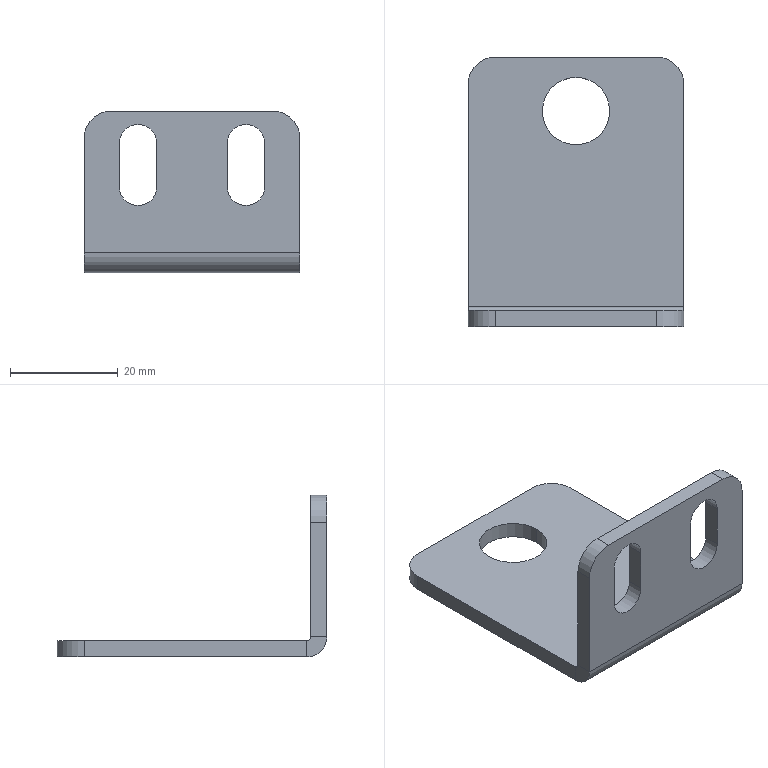Part | SolidWorks | features BaseBody 1 | 1 solid | 30 faces | box 40 x 50 x 30 mm | volume 8125 mm3 | plane 16 | cylinder 14 | commonest cylinder face diameters 7 x6 10 x4 12.5 x2 1.473 x1 7.473 x1
STEP:
#1=CARTESIAN_POINT('',(10.,-26.5,24.5));
#2=VERTEX_POINT('',#1);
#3=CARTESIAN_POINT('',(13.5,-26.5,21.));
#4=VERTEX_POINT('',#3);
#5=CARTESIAN_POINT('',(10.,-26.5,21.));
#6=DIRECTION('',(0.,1.,0.));
#7=DIRECTION('',(0.,0.,1.));
#8=AXIS2_PLACEMENT_3D('',#5,#6,#7);
#9=CIRCLE('',#8,3.5);
#10=EDGE_CURVE('',#2,#4,#9,.T.);
#11=ORIENTED_EDGE('',*,*,#10,.F.);
#12=CARTESIAN_POINT('',(10.,-23.5,24.5));
#13=VERTEX_POINT('',#12);
#14=CARTESIAN_POINT('',(10.,-33.5,24.5));
#15=DIRECTION('',(0.,1.,0.));
#16=VECTOR('',#15,1000.);
#17=LINE('',#14,#16);
#18=EDGE_CURVE('',#2,#13,#17,.T.);
#19=ORIENTED_EDGE('',*,*,#18,.T.);
#20=CARTESIAN_POINT('',(13.5,-23.5,21.));
#21=VERTEX_POINT('',#20);
#22=CARTESIAN_POINT('',(10.,-23.5,21.));
#23=DIRECTION('',(0.,1.,0.));
#24=DIRECTION('',(0.,0.,1.));
#25=AXIS2_PLACEMENT_3D('',#22,#23,#24);
#26=CIRCLE('',#25,3.5);
#27=EDGE_CURVE('',#13,#21,#26,.T.);
#28=ORIENTED_EDGE('',*,*,#27,.T.);
#29=CARTESIAN_POINT('',(13.5,-33.5,21.));
#30=DIRECTION('',(0.,1.,0.));
#31=VECTOR('',#30,1000.);
#32=LINE('',#29,#31);
#33=EDGE_CURVE('',#4,#21,#32,.T.);
#34=ORIENTED_EDGE('',*,*,#33,.F.);
#35=EDGE_LOOP('',(#11,#19,#28,#34));
#36=FACE_OUTER_BOUND('',#35,.T.);
#37=CARTESIAN_POINT('',(10.,-33.5,21.));
#38=DIRECTION('',(0.,1.,0.));
#39=DIRECTION('',(0.,0.,1.));
#40=AXIS2_PLACEMENT_3D('',#37,#38,#39);
#41=CYLINDRICAL_SURFACE('',#40,3.5);
#42=ADVANCED_FACE('',(#36),#41,.F.);
#43=CARTESIAN_POINT('',(-10.,-26.5,24.5));
#44=VERTEX_POINT('',#43);
#45=CARTESIAN_POINT('',(-6.5,-26.5,21.));
#46=VERTEX_POINT('',#45);
#47=CARTESIAN_POINT('',(-10.,-26.5,21.));
#48=DIRECTION('',(0.,1.,0.));
#49=DIRECTION('',(0.,0.,1.));
#50=AXIS2_PLACEMENT_3D('',#47,#48,#49);
#51=CIRCLE('',#50,3.5);
#52=EDGE_CURVE('',#44,#46,#51,.T.);
#53=ORIENTED_EDGE('',*,*,#52,.F.);
#54=CARTESIAN_POINT('',(-10.,-23.5,24.5));
#55=VERTEX_POINT('',#54);
#56=CARTESIAN_POINT('',(-10.,-33.5,24.5));
#57=DIRECTION('',(0.,1.,0.));
#58=VECTOR('',#57,1000.);
#59=LINE('',#56,#58);
#60=EDGE_CURVE('',#44,#55,#59,.T.);
#61=ORIENTED_EDGE('',*,*,#60,.T.);
#62=CARTESIAN_POINT('',(-6.5,-23.5,21.));
#63=VERTEX_POINT('',#62);
#64=CARTESIAN_POINT('',(-10.,-23.5,21.));
#65=DIRECTION('',(0.,1.,0.));
#66=DIRECTION('',(0.,0.,1.));
#67=AXIS2_PLACEMENT_3D('',#64,#65,#66);
#68=CIRCLE('',#67,3.5);
#69=EDGE_CURVE('',#55,#63,#68,.T.);
#70=ORIENTED_EDGE('',*,*,#69,.T.);
#71=CARTESIAN_POINT('',(-6.5,-33.5,21.));
#72=DIRECTION('',(0.,1.,0.));
#73=VECTOR('',#72,1000.);
#74=LINE('',#71,#73);
#75=EDGE_CURVE('',#46,#63,#74,.T.);
#76=ORIENTED_EDGE('',*,*,#75,.F.);
#77=EDGE_LOOP('',(#53,#61,#70,#76));
#78=FACE_OUTER_BOUND('',#77,.T.);
#79=CARTESIAN_POINT('',(-10.,-33.5,21.));
#80=DIRECTION('',(0.,1.,0.));
#81=DIRECTION('',(0.,0.,1.));
#82=AXIS2_PLACEMENT_3D('',#79,#80,#81);
#83=CYLINDRICAL_SURFACE('',#82,3.5);
#84=ADVANCED_FACE('',(#78),#83,.F.);
#85=CARTESIAN_POINT('',(-6.25,13.5,0.));
#86=VERTEX_POINT('',#85);
#87=CARTESIAN_POINT('',(6.25,13.5,0.));
#88=VERTEX_POINT('',#87);
#89=CARTESIAN_POINT('',(0.,13.5,0.));
#90=DIRECTION('',(0.,0.,1.));
#91=DIRECTION('',(1.,0.,0.));
#92=AXIS2_PLACEMENT_3D('',#89,#90,#91);
#93=CIRCLE('',#92,6.25);
#94=EDGE_CURVE('',#86,#88,#93,.T.);
#95=ORIENTED_EDGE('',*,*,#94,.T.);
#96=CARTESIAN_POINT('',(6.25,13.5,-3.));
#97=VERTEX_POINT('',#96);
#98=CARTESIAN_POINT('',(6.25,13.5,-3.));
#99=DIRECTION('',(0.,0.,-1.));
#100=VECTOR('',#99,1000.);
#101=LINE('',#98,#100);
#102=EDGE_CURVE('',#88,#97,#101,.T.);
#103=ORIENTED_EDGE('',*,*,#102,.T.);
#104=CARTESIAN_POINT('',(-6.25,13.5,-3.));
#105=VERTEX_POINT('',#104);
#106=CARTESIAN_POINT('',(0.,13.5,-3.));
#107=DIRECTION('',(0.,0.,-1.));
#108=DIRECTION('',(-1.,0.,0.));
#109=AXIS2_PLACEMENT_3D('',#106,#107,#108);
#110=CIRCLE('',#109,6.25);
#111=EDGE_CURVE('',#97,#105,#110,.T.);
#112=ORIENTED_EDGE('',*,*,#111,.T.);
#113=CARTESIAN_POINT('',(-6.25,13.5,-3.));
#114=DIRECTION('',(0.,0.,-1.));
#115=VECTOR('',#114,1000.);
#116=LINE('',#113,#115);
#117=EDGE_CURVE('',#86,#105,#116,.T.);
#118=ORIENTED_EDGE('',*,*,#117,.F.);
#119=EDGE_LOOP('',(#95,#103,#112,#118));
#120=FACE_OUTER_BOUND('',#119,.T.);
#121=CARTESIAN_POINT('',(0.,13.5,-3.));
#122=DIRECTION('',(0.,0.,-1.));
#123=DIRECTION('',(-1.,0.,0.));
#124=AXIS2_PLACEMENT_3D('',#121,#122,#123);
#125=CYLINDRICAL_SURFACE('',#124,6.25);
#126=ADVANCED_FACE('',(#120),#125,.F.);
#127=CARTESIAN_POINT('',(20.,-22.763,-3.));
#128=VERTEX_POINT('',#127);
#129=CARTESIAN_POINT('',(20.,18.5,-3.));
#130=VERTEX_POINT('',#129);
#131=CARTESIAN_POINT('',(20.,23.5,-3.));
#132=DIRECTION('',(0.,1.,0.));
#133=VECTOR('',#132,1000.);
#134=LINE('',#131,#133);
#135=EDGE_CURVE('',#128,#130,#134,.T.);
#136=ORIENTED_EDGE('',*,*,#135,.T.);
#137=CARTESIAN_POINT('',(20.,18.5,0.));
#138=VERTEX_POINT('',#137);
#139=CARTESIAN_POINT('',(20.,18.5,-3.));
#140=DIRECTION('',(0.,0.,1.));
#141=VECTOR('',#140,1000.);
#142=LINE('',#139,#141);
#143=EDGE_CURVE('',#130,#138,#142,.T.);
#144=ORIENTED_EDGE('',*,*,#143,.T.);
#145=CARTESIAN_POINT('',(20.,-22.763,0.));
#146=VERTEX_POINT('',#145);
#147=CARTESIAN_POINT('',(20.,23.5,0.));
#148=DIRECTION('',(0.,1.,0.));
#149=VECTOR('',#148,1000.);
#150=LINE('',#147,#149);
#151=EDGE_CURVE('',#146,#138,#150,.T.);
#152=ORIENTED_EDGE('',*,*,#151,.F.);
#153=CARTESIAN_POINT('',(20.,-22.763,0.));
#154=DIRECTION('',(0.,0.,-1.));
#155=VECTOR('',#154,1000.);
#156=LINE('',#153,#155);
#157=EDGE_CURVE('',#146,#128,#156,.T.);
#158=ORIENTED_EDGE('',*,*,#157,.T.);
#159=EDGE_LOOP('',(#136,#144,#152,#158));
#160=FACE_OUTER_BOUND('',#159,.T.);
#161=CARTESIAN_POINT('',(20.,23.5,-3.));
#162=DIRECTION('',(1.,0.,0.));
#163=DIRECTION('',(0.,1.,0.));
#164=AXIS2_PLACEMENT_3D('',#161,#162,#163);
#165=PLANE('',#164);
#166=ADVANCED_FACE('',(#160),#165,.T.);
#167=CARTESIAN_POINT('',(0.,13.5,-3.));
#168=DIRECTION('',(0.,0.,-1.));
#169=DIRECTION('',(-1.,0.,0.));
#170=AXIS2_PLACEMENT_3D('',#167,#168,#169);
#171=CIRCLE('',#170,6.25);
#172=EDGE_CURVE('',#105,#97,#171,.T.);
#173=ORIENTED_EDGE('',*,*,#172,.F.);
#174=ORIENTED_EDGE('',*,*,#111,.F.);
#175=EDGE_LOOP('',(#173,#174));
#176=FACE_BOUND('',#175,.T.);
#177=CARTESIAN_POINT('',(15.,23.5,-3.));
#178=VERTEX_POINT('',#177);
#179=CARTESIAN_POINT('',(-15.,23.5,-3.));
#180=VERTEX_POINT('',#179);
#181=CARTESIAN_POINT('',(-20.,23.5,-3.));
#182=DIRECTION('',(-1.,0.,0.));
#183=VECTOR('',#182,1000.);
#184=LINE('',#181,#183);
#185=EDGE_CURVE('',#178,#180,#184,.T.);
#186=ORIENTED_EDGE('',*,*,#185,.F.);
#187=CARTESIAN_POINT('',(15.,18.5,-3.));
#188=DIRECTION('',(0.,0.,-1.));
#189=DIRECTION('',(1.,0.,0.));
#190=AXIS2_PLACEMENT_3D('',#187,#188,#189);
#191=CIRCLE('',#190,5.);
#192=EDGE_CURVE('',#178,#130,#191,.T.);
#193=ORIENTED_EDGE('',*,*,#192,.T.);
#194=ORIENTED_EDGE('',*,*,#135,.F.);
#195=CARTESIAN_POINT('',(-20.,-22.763,-3.));
#196=VERTEX_POINT('',#195);
#197=CARTESIAN_POINT('',(20.,-22.763,-3.));
#198=DIRECTION('',(-1.,0.,0.));
#199=VECTOR('',#198,1000.);
#200=LINE('',#197,#199);
#201=EDGE_CURVE('',#128,#196,#200,.T.);
#202=ORIENTED_EDGE('',*,*,#201,.T.);
#203=CARTESIAN_POINT('',(-20.,18.5,-3.));
#204=VERTEX_POINT('',#203);
#205=CARTESIAN_POINT('',(-20.,23.5,-3.));
#206=DIRECTION('',(0.,-1.,0.));
#207=VECTOR('',#206,1000.);
#208=LINE('',#205,#207);
#209=EDGE_CURVE('',#204,#196,#208,.T.);
#210=ORIENTED_EDGE('',*,*,#209,.F.);
#211=CARTESIAN_POINT('',(-15.,18.5,-3.));
#212=DIRECTION('',(0.,0.,-1.));
#213=DIRECTION('',(1.,0.,0.));
#214=AXIS2_PLACEMENT_3D('',#211,#212,#213);
#215=CIRCLE('',#214,5.);
#216=EDGE_CURVE('',#204,#180,#215,.T.);
#217=ORIENTED_EDGE('',*,*,#216,.T.);
#218=EDGE_LOOP('',(#186,#193,#194,#202,#210,#217));
#219=FACE_OUTER_BOUND('',#218,.T.);
#220=CARTESIAN_POINT('',(0.,0.,-3.));
#221=DIRECTION('',(0.,0.,1.));
#222=DIRECTION('',(1.,0.,0.));
#223=AXIS2_PLACEMENT_3D('',#220,#221,#222);
#224=PLANE('',#223);
#225=ADVANCED_FACE('',(#176,#219),#224,.F.);
#226=ORIENTED_EDGE('',*,*,#94,.F.);
#227=CARTESIAN_POINT('',(0.,13.5,0.));
#228=DIRECTION('',(0.,0.,1.));
#229=DIRECTION('',(1.,0.,0.));
#230=AXIS2_PLACEMENT_3D('',#227,#228,#229);
#231=CIRCLE('',#230,6.25);
#232=EDGE_CURVE('',#88,#86,#231,.T.);
#233=ORIENTED_EDGE('',*,*,#232,.F.);
#234=EDGE_LOOP('',(#226,#233));
#235=FACE_BOUND('',#234,.T.);
#236=ORIENTED_EDGE('',*,*,#151,.T.);
#237=CARTESIAN_POINT('',(15.,23.5,0.));
#238=VERTEX_POINT('',#237);
#239=CARTESIAN_POINT('',(15.,18.5,0.));
#240=DIRECTION('',(0.,0.,1.));
#241=DIRECTION('',(1.,0.,0.));
#242=AXIS2_PLACEMENT_3D('',#239,#240,#241);
#243=CIRCLE('',#242,5.);
#244=EDGE_CURVE('',#138,#238,#243,.T.);
#245=ORIENTED_EDGE('',*,*,#244,.T.);
#246=CARTESIAN_POINT('',(-15.,23.5,0.));
#247=VERTEX_POINT('',#246);
#248=CARTESIAN_POINT('',(-20.,23.5,0.));
#249=DIRECTION('',(-1.,0.,0.));
#250=VECTOR('',#249,1000.);
#251=LINE('',#248,#250);
#252=EDGE_CURVE('',#238,#247,#251,.T.);
#253=ORIENTED_EDGE('',*,*,#252,.T.);
#254=CARTESIAN_POINT('',(-20.,18.5,0.));
#255=VERTEX_POINT('',#254);
#256=CARTESIAN_POINT('',(-15.,18.5,0.));
#257=DIRECTION('',(0.,0.,1.));
#258=DIRECTION('',(1.,0.,0.));
#259=AXIS2_PLACEMENT_3D('',#256,#257,#258);
#260=CIRCLE('',#259,5.);
#261=EDGE_CURVE('',#247,#255,#260,.T.);
#262=ORIENTED_EDGE('',*,*,#261,.T.);
#263=CARTESIAN_POINT('',(-20.,-22.763,0.));
#264=VERTEX_POINT('',#263);
#265=CARTESIAN_POINT('',(-20.,23.5,0.));
#266=DIRECTION('',(0.,-1.,0.));
#267=VECTOR('',#266,1000.);
#268=LINE('',#265,#267);
#269=EDGE_CURVE('',#255,#264,#268,.T.);
#270=ORIENTED_EDGE('',*,*,#269,.T.);
#271=CARTESIAN_POINT('',(20.,-22.763,0.));
#272=DIRECTION('',(-1.,0.,0.));
#273=VECTOR('',#272,1000.);
#274=LINE('',#271,#273);
#275=EDGE_CURVE('',#146,#264,#274,.T.);
#276=ORIENTED_EDGE('',*,*,#275,.F.);
#277=EDGE_LOOP('',(#236,#245,#253,#262,#270,#276));
#278=FACE_OUTER_BOUND('',#277,.T.);
#279=CARTESIAN_POINT('',(0.,0.,0.));
#280=DIRECTION('',(0.,0.,1.));
#281=DIRECTION('',(1.,0.,0.));
#282=AXIS2_PLACEMENT_3D('',#279,#280,#281);
#283=PLANE('',#282);
#284=ADVANCED_FACE('',(#235,#278),#283,.T.);
#285=ORIENTED_EDGE('',*,*,#269,.F.);
#286=CARTESIAN_POINT('',(-20.,18.5,-3.));
#287=DIRECTION('',(0.,0.,-1.));
#288=VECTOR('',#287,1000.);
#289=LINE('',#286,#288);
#290=EDGE_CURVE('',#255,#204,#289,.T.);
#291=ORIENTED_EDGE('',*,*,#290,.T.);
#292=ORIENTED_EDGE('',*,*,#209,.T.);
#293=CARTESIAN_POINT('',(-20.,-22.763,0.));
#294=DIRECTION('',(0.,0.,-1.));
#295=VECTOR('',#294,1000.);
#296=LINE('',#293,#295);
#297=EDGE_CURVE('',#264,#196,#296,.T.);
#298=ORIENTED_EDGE('',*,*,#297,.F.);
#299=EDGE_LOOP('',(#285,#291,#292,#298));
#300=FACE_OUTER_BOUND('',#299,.T.);
#301=CARTESIAN_POINT('',(-20.,23.5,-3.));
#302=DIRECTION('',(-1.,0.,0.));
#303=DIRECTION('',(0.,-1.,0.));
#304=AXIS2_PLACEMENT_3D('',#301,#302,#303);
#305=PLANE('',#304);
#306=ADVANCED_FACE('',(#300),#305,.T.);
#307=ORIENTED_EDGE('',*,*,#252,.F.);
#308=CARTESIAN_POINT('',(15.,23.5,-3.));
#309=DIRECTION('',(0.,0.,-1.));
#310=VECTOR('',#309,1000.);
#311=LINE('',#308,#310);
#312=EDGE_CURVE('',#238,#178,#311,.T.);
#313=ORIENTED_EDGE('',*,*,#312,.T.);
#314=ORIENTED_EDGE('',*,*,#185,.T.);
#315=CARTESIAN_POINT('',(-15.,23.5,-3.));
#316=DIRECTION('',(0.,0.,1.));
#317=VECTOR('',#316,1000.);
#318=LINE('',#315,#317);
#319=EDGE_CURVE('',#180,#247,#318,.T.);
#320=ORIENTED_EDGE('',*,*,#319,.T.);
#321=EDGE_LOOP('',(#307,#313,#314,#320));
#322=FACE_OUTER_BOUND('',#321,.T.);
#323=CARTESIAN_POINT('',(-20.,23.5,-3.));
#324=DIRECTION('',(0.,1.,0.));
#325=DIRECTION('',(0.,0.,1.));
#326=AXIS2_PLACEMENT_3D('',#323,#324,#325);
#327=PLANE('',#326);
#328=ADVANCED_FACE('',(#322),#327,.T.);
#329=CARTESIAN_POINT('',(-20.,-23.5,0.7366));
#330=VERTEX_POINT('',#329);
#331=CARTESIAN_POINT('',(-20.,-26.5,0.7366));
#332=VERTEX_POINT('',#331);
#333=CARTESIAN_POINT('',(-20.,-23.5,0.7366));
#334=DIRECTION('',(0.,-1.,0.));
#335=VECTOR('',#334,1000.);
#336=LINE('',#333,#335);
#337=EDGE_CURVE('',#330,#332,#336,.T.);
#338=ORIENTED_EDGE('',*,*,#337,.F.);
#339=CARTESIAN_POINT('',(-20.,-22.763,0.7366));
#340=DIRECTION('',(-1.,0.,0.));
#341=DIRECTION('',(0.,0.,-1.));
#342=AXIS2_PLACEMENT_3D('',#339,#340,#341);
#343=CIRCLE('',#342,0.7366);
#344=EDGE_CURVE('',#264,#330,#343,.T.);
#345=ORIENTED_EDGE('',*,*,#344,.F.);
#346=ORIENTED_EDGE('',*,*,#297,.T.);
#347=CARTESIAN_POINT('',(-20.,-22.763,0.7366));
#348=DIRECTION('',(-1.,0.,0.));
#349=DIRECTION('',(0.,0.,-1.));
#350=AXIS2_PLACEMENT_3D('',#347,#348,#349);
#351=CIRCLE('',#350,3.737);
#352=EDGE_CURVE('',#196,#332,#351,.T.);
#353=ORIENTED_EDGE('',*,*,#352,.T.);
#354=EDGE_LOOP('',(#338,#345,#346,#353));
#355=FACE_OUTER_BOUND('',#354,.T.);
#356=CARTESIAN_POINT('',(-20.,-22.763,0.7366));
#357=DIRECTION('',(-1.,0.,0.));
#358=DIRECTION('',(0.,0.,1.));
#359=AXIS2_PLACEMENT_3D('',#356,#357,#358);
#360=PLANE('',#359);
#361=ADVANCED_FACE('',(#355),#360,.T.);
#362=CARTESIAN_POINT('',(20.,-23.5,0.7366));
#363=VERTEX_POINT('',#362);
#364=CARTESIAN_POINT('',(20.,-22.763,0.7366));
#365=DIRECTION('',(1.,0.,0.));
#366=DIRECTION('',(0.,0.,-1.));
#367=AXIS2_PLACEMENT_3D('',#364,#365,#366);
#368=CIRCLE('',#367,0.7366);
#369=EDGE_CURVE('',#363,#146,#368,.T.);
#370=ORIENTED_EDGE('',*,*,#369,.F.);
#371=CARTESIAN_POINT('',(20.,-26.5,0.7366));
#372=VERTEX_POINT('',#371);
#373=CARTESIAN_POINT('',(20.,-23.5,0.7366));
#374=DIRECTION('',(0.,-1.,0.));
#375=VECTOR('',#374,1000.);
#376=LINE('',#373,#375);
#377=EDGE_CURVE('',#363,#372,#376,.T.);
#378=ORIENTED_EDGE('',*,*,#377,.T.);
#379=CARTESIAN_POINT('',(20.,-22.763,0.7366));
#380=DIRECTION('',(1.,0.,0.));
#381=DIRECTION('',(0.,0.,-1.));
#382=AXIS2_PLACEMENT_3D('',#379,#380,#381);
#383=CIRCLE('',#382,3.737);
#384=EDGE_CURVE('',#372,#128,#383,.T.);
#385=ORIENTED_EDGE('',*,*,#384,.T.);
#386=ORIENTED_EDGE('',*,*,#157,.F.);
#387=EDGE_LOOP('',(#370,#378,#385,#386));
#388=FACE_OUTER_BOUND('',#387,.T.);
#389=CARTESIAN_POINT('',(20.,-22.763,0.7366));
#390=DIRECTION('',(-1.,0.,0.));
#391=DIRECTION('',(0.,0.,1.));
#392=AXIS2_PLACEMENT_3D('',#389,#390,#391);
#393=PLANE('',#392);
#394=ADVANCED_FACE('',(#388),#393,.F.);
#395=ORIENTED_EDGE('',*,*,#201,.F.);
#396=ORIENTED_EDGE('',*,*,#384,.F.);
#397=CARTESIAN_POINT('',(0.,-26.5,0.7366));
#398=DIRECTION('',(-1.,0.,0.));
#399=VECTOR('',#398,1000.);
#400=LINE('',#397,#399);
#401=EDGE_CURVE('',#372,#332,#400,.T.);
#402=ORIENTED_EDGE('',*,*,#401,.T.);
#403=ORIENTED_EDGE('',*,*,#352,.F.);
#404=EDGE_LOOP('',(#395,#396,#402,#403));
#405=FACE_OUTER_BOUND('',#404,.T.);
#406=CARTESIAN_POINT('',(20.,-22.763,0.7366));
#407=DIRECTION('',(1.,0.,0.));
#408=DIRECTION('',(0.,-1.,0.));
#409=AXIS2_PLACEMENT_3D('',#406,#407,#408);
#410=CYLINDRICAL_SURFACE('',#409,3.737);
#411=ADVANCED_FACE('',(#405),#410,.T.);
#412=ORIENTED_EDGE('',*,*,#275,.T.);
#413=ORIENTED_EDGE('',*,*,#344,.T.);
#414=CARTESIAN_POINT('',(-20.,-23.5,0.7366));
#415=DIRECTION('',(1.,0.,0.));
#416=VECTOR('',#415,1000.);
#417=LINE('',#414,#416);
#418=EDGE_CURVE('',#330,#363,#417,.T.);
#419=ORIENTED_EDGE('',*,*,#418,.T.);
#420=ORIENTED_EDGE('',*,*,#369,.T.);
#421=EDGE_LOOP('',(#412,#413,#419,#420));
#422=FACE_OUTER_BOUND('',#421,.T.);
#423=CARTESIAN_POINT('',(20.,-22.763,0.7366));
#424=DIRECTION('',(1.,0.,0.));
#425=DIRECTION('',(0.,-1.,0.));
#426=AXIS2_PLACEMENT_3D('',#423,#424,#425);
#427=CYLINDRICAL_SURFACE('',#426,0.7366);
#428=ADVANCED_FACE('',(#422),#427,.F.);
#429=CARTESIAN_POINT('',(-20.,-26.5,22.));
#430=VERTEX_POINT('',#429);
#431=CARTESIAN_POINT('',(-20.,-26.5,0.));
#432=DIRECTION('',(0.,0.,-1.));
#433=VECTOR('',#432,1000.);
#434=LINE('',#431,#433);
#435=EDGE_CURVE('',#430,#332,#434,.T.);
#436=ORIENTED_EDGE('',*,*,#435,.F.);
#437=CARTESIAN_POINT('',(-20.,-23.5,22.));
#438=VERTEX_POINT('',#437);
#439=CARTESIAN_POINT('',(-20.,-26.5,22.));
#440=DIRECTION('',(0.,1.,0.));
#441=VECTOR('',#440,1000.);
#442=LINE('',#439,#441);
#443=EDGE_CURVE('',#430,#438,#442,.T.);
#444=ORIENTED_EDGE('',*,*,#443,.T.);
#445=CARTESIAN_POINT('',(-20.,-23.5,0.));
#446=DIRECTION('',(0.,0.,-1.));
#447=VECTOR('',#446,1000.);
#448=LINE('',#445,#447);
#449=EDGE_CURVE('',#438,#330,#448,.T.);
#450=ORIENTED_EDGE('',*,*,#449,.T.);
#451=ORIENTED_EDGE('',*,*,#337,.T.);
#452=EDGE_LOOP('',(#436,#444,#450,#451));
#453=FACE_OUTER_BOUND('',#452,.T.);
#454=CARTESIAN_POINT('',(-20.,-26.5,0.));
#455=DIRECTION('',(1.,0.,0.));
#456=DIRECTION('',(0.,0.,-1.));
#457=AXIS2_PLACEMENT_3D('',#454,#455,#456);
#458=PLANE('',#457);
#459=ADVANCED_FACE('',(#453),#458,.F.);
#460=CARTESIAN_POINT('',(20.,-23.5,22.));
#461=VERTEX_POINT('',#460);
#462=CARTESIAN_POINT('',(20.,-23.5,27.));
#463=DIRECTION('',(0.,0.,1.));
#464=VECTOR('',#463,1000.);
#465=LINE('',#462,#464);
#466=EDGE_CURVE('',#363,#461,#465,.T.);
#467=ORIENTED_EDGE('',*,*,#466,.T.);
#468=CARTESIAN_POINT('',(20.,-26.5,22.));
#469=VERTEX_POINT('',#468);
#470=CARTESIAN_POINT('',(20.,-26.5,22.));
#471=DIRECTION('',(0.,-1.,0.));
#472=VECTOR('',#471,1000.);
#473=LINE('',#470,#472);
#474=EDGE_CURVE('',#461,#469,#473,.T.);
#475=ORIENTED_EDGE('',*,*,#474,.T.);
#476=CARTESIAN_POINT('',(20.,-26.5,27.));
#477=DIRECTION('',(0.,0.,1.));
#478=VECTOR('',#477,1000.);
#479=LINE('',#476,#478);
#480=EDGE_CURVE('',#372,#469,#479,.T.);
#481=ORIENTED_EDGE('',*,*,#480,.F.);
#482=ORIENTED_EDGE('',*,*,#377,.F.);
#483=EDGE_LOOP('',(#467,#475,#481,#482));
#484=FACE_OUTER_BOUND('',#483,.T.);
#485=CARTESIAN_POINT('',(20.,-26.5,27.));
#486=DIRECTION('',(-1.,0.,0.));
#487=DIRECTION('',(0.,0.,1.));
#488=AXIS2_PLACEMENT_3D('',#485,#486,#487);
#489=PLANE('',#488);
#490=ADVANCED_FACE('',(#484),#489,.F.);
#491=CARTESIAN_POINT('',(13.5,-26.5,13.));
#492=VERTEX_POINT('',#491);
#493=CARTESIAN_POINT('',(13.5,-26.5,0.));
#494=DIRECTION('',(0.,0.,-1.));
#495=VECTOR('',#494,1000.);
#496=LINE('',#493,#495);
#497=EDGE_CURVE('',#4,#492,#496,.T.);
#498=ORIENTED_EDGE('',*,*,#497,.T.);
#499=CARTESIAN_POINT('',(6.5,-26.5,13.));
#500=VERTEX_POINT('',#499);
#501=CARTESIAN_POINT('',(10.,-26.5,13.));
#502=DIRECTION('',(0.,1.,0.));
#503=DIRECTION('',(0.,0.,1.));
#504=AXIS2_PLACEMENT_3D('',#501,#502,#503);
#505=CIRCLE('',#504,3.5);
#506=EDGE_CURVE('',#492,#500,#505,.T.);
#507=ORIENTED_EDGE('',*,*,#506,.T.);
#508=CARTESIAN_POINT('',(6.5,-26.5,21.));
#509=VERTEX_POINT('',#508);
#510=CARTESIAN_POINT('',(6.5,-26.5,0.));
#511=DIRECTION('',(0.,0.,1.));
#512=VECTOR('',#511,1000.);
#513=LINE('',#510,#512);
#514=EDGE_CURVE('',#500,#509,#513,.T.);
#515=ORIENTED_EDGE('',*,*,#514,.T.);
#516=CARTESIAN_POINT('',(10.,-26.5,21.));
#517=DIRECTION('',(0.,1.,0.));
#518=DIRECTION('',(0.,0.,1.));
#519=AXIS2_PLACEMENT_3D('',#516,#517,#518);
#520=CIRCLE('',#519,3.5);
#521=EDGE_CURVE('',#509,#2,#520,.T.);
#522=ORIENTED_EDGE('',*,*,#521,.T.);
#523=ORIENTED_EDGE('',*,*,#10,.T.);
#524=EDGE_LOOP('',(#498,#507,#515,#522,#523));
#525=FACE_BOUND('',#524,.T.);
#526=CARTESIAN_POINT('',(-6.5,-26.5,13.));
#527=VERTEX_POINT('',#526);
#528=CARTESIAN_POINT('',(-6.5,-26.5,0.));
#529=DIRECTION('',(0.,0.,-1.));
#530=VECTOR('',#529,1000.);
#531=LINE('',#528,#530);
#532=EDGE_CURVE('',#46,#527,#531,.T.);
#533=ORIENTED_EDGE('',*,*,#532,.T.);
#534=CARTESIAN_POINT('',(-13.5,-26.5,13.));
#535=VERTEX_POINT('',#534);
#536=CARTESIAN_POINT('',(-10.,-26.5,13.));
#537=DIRECTION('',(0.,1.,0.));
#538=DIRECTION('',(0.,0.,1.));
#539=AXIS2_PLACEMENT_3D('',#536,#537,#538);
#540=CIRCLE('',#539,3.5);
#541=EDGE_CURVE('',#527,#535,#540,.T.);
#542=ORIENTED_EDGE('',*,*,#541,.T.);
#543=CARTESIAN_POINT('',(-13.5,-26.5,21.));
#544=VERTEX_POINT('',#543);
#545=CARTESIAN_POINT('',(-13.5,-26.5,0.));
#546=DIRECTION('',(0.,0.,1.));
#547=VECTOR('',#546,1000.);
#548=LINE('',#545,#547);
#549=EDGE_CURVE('',#535,#544,#548,.T.);
#550=ORIENTED_EDGE('',*,*,#549,.T.);
#551=CARTESIAN_POINT('',(-10.,-26.5,21.));
#552=DIRECTION('',(0.,1.,0.));
#553=DIRECTION('',(0.,0.,1.));
#554=AXIS2_PLACEMENT_3D('',#551,#552,#553);
#555=CIRCLE('',#554,3.5);
#556=EDGE_CURVE('',#544,#44,#555,.T.);
#557=ORIENTED_EDGE('',*,*,#556,.T.);
#558=ORIENTED_EDGE('',*,*,#52,.T.);
#559=EDGE_LOOP('',(#533,#542,#550,#557,#558));
#560=FACE_BOUND('',#559,.T.);
#561=CARTESIAN_POINT('',(15.,-26.5,27.));
#562=VERTEX_POINT('',#561);
#563=CARTESIAN_POINT('',(-15.,-26.5,27.));
#564=VERTEX_POINT('',#563);
#565=CARTESIAN_POINT('',(-20.,-26.5,27.));
#566=DIRECTION('',(-1.,0.,0.));
#567=VECTOR('',#566,1000.);
#568=LINE('',#565,#567);
#569=EDGE_CURVE('',#562,#564,#568,.T.);
#570=ORIENTED_EDGE('',*,*,#569,.T.);
#571=CARTESIAN_POINT('',(-15.,-26.5,22.));
#572=DIRECTION('',(0.,-1.,0.));
#573=DIRECTION('',(0.,0.,1.));
#574=AXIS2_PLACEMENT_3D('',#571,#572,#573);
#575=CIRCLE('',#574,5.);
#576=EDGE_CURVE('',#564,#430,#575,.T.);
#577=ORIENTED_EDGE('',*,*,#576,.T.);
#578=ORIENTED_EDGE('',*,*,#435,.T.);
#579=ORIENTED_EDGE('',*,*,#401,.F.);
#580=ORIENTED_EDGE('',*,*,#480,.T.);
#581=CARTESIAN_POINT('',(15.,-26.5,22.));
#582=DIRECTION('',(0.,-1.,0.));
#583=DIRECTION('',(0.,0.,1.));
#584=AXIS2_PLACEMENT_3D('',#581,#582,#583);
#585=CIRCLE('',#584,5.);
#586=EDGE_CURVE('',#469,#562,#585,.T.);
#587=ORIENTED_EDGE('',*,*,#586,.T.);
#588=EDGE_LOOP('',(#570,#577,#578,#579,#580,#587));
#589=FACE_OUTER_BOUND('',#588,.T.);
#590=CARTESIAN_POINT('',(0.,-26.5,0.));
#591=DIRECTION('',(0.,1.,0.));
#592=DIRECTION('',(0.,0.,1.));
#593=AXIS2_PLACEMENT_3D('',#590,#591,#592);
#594=PLANE('',#593);
#595=ADVANCED_FACE('',(#525,#560,#589),#594,.F.);
#596=CARTESIAN_POINT('',(13.5,-23.5,13.));
#597=VERTEX_POINT('',#596);
#598=CARTESIAN_POINT('',(6.5,-23.5,13.));
#599=VERTEX_POINT('',#598);
#600=CARTESIAN_POINT('',(10.,-23.5,13.));
#601=DIRECTION('',(0.,1.,0.));
#602=DIRECTION('',(0.,0.,1.));
#603=AXIS2_PLACEMENT_3D('',#600,#601,#602);
#604=CIRCLE('',#603,3.5);
#605=EDGE_CURVE('',#597,#599,#604,.T.);
#606=ORIENTED_EDGE('',*,*,#605,.F.);
#607=CARTESIAN_POINT('',(13.5,-23.5,13.));
#608=DIRECTION('',(0.,0.,-1.));
#609=VECTOR('',#608,1000.);
#610=LINE('',#607,#609);
#611=EDGE_CURVE('',#21,#597,#610,.T.);
#612=ORIENTED_EDGE('',*,*,#611,.F.);
#613=ORIENTED_EDGE('',*,*,#27,.F.);
#614=CARTESIAN_POINT('',(6.5,-23.5,21.));
#615=VERTEX_POINT('',#614);
#616=CARTESIAN_POINT('',(10.,-23.5,21.));
#617=DIRECTION('',(0.,1.,0.));
#618=DIRECTION('',(0.,0.,1.));
#619=AXIS2_PLACEMENT_3D('',#616,#617,#618);
#620=CIRCLE('',#619,3.5);
#621=EDGE_CURVE('',#615,#13,#620,.T.);
#622=ORIENTED_EDGE('',*,*,#621,.F.);
#623=CARTESIAN_POINT('',(6.5,-23.5,13.));
#624=DIRECTION('',(0.,0.,1.));
#625=VECTOR('',#624,1000.);
#626=LINE('',#623,#625);
#627=EDGE_CURVE('',#599,#615,#626,.T.);
#628=ORIENTED_EDGE('',*,*,#627,.F.);
#629=EDGE_LOOP('',(#606,#612,#613,#622,#628));
#630=FACE_BOUND('',#629,.T.);
#631=CARTESIAN_POINT('',(-6.5,-23.5,13.));
#632=VERTEX_POINT('',#631);
#633=CARTESIAN_POINT('',(-13.5,-23.5,13.));
#634=VERTEX_POINT('',#633);
#635=CARTESIAN_POINT('',(-10.,-23.5,13.));
#636=DIRECTION('',(0.,1.,0.));
#637=DIRECTION('',(0.,0.,1.));
#638=AXIS2_PLACEMENT_3D('',#635,#636,#637);
#639=CIRCLE('',#638,3.5);
#640=EDGE_CURVE('',#632,#634,#639,.T.);
#641=ORIENTED_EDGE('',*,*,#640,.F.);
#642=CARTESIAN_POINT('',(-6.5,-23.5,13.));
#643=DIRECTION('',(0.,0.,-1.));
#644=VECTOR('',#643,1000.);
#645=LINE('',#642,#644);
#646=EDGE_CURVE('',#63,#632,#645,.T.);
#647=ORIENTED_EDGE('',*,*,#646,.F.);
#648=ORIENTED_EDGE('',*,*,#69,.F.);
#649=CARTESIAN_POINT('',(-13.5,-23.5,21.));
#650=VERTEX_POINT('',#649);
#651=CARTESIAN_POINT('',(-10.,-23.5,21.));
#652=DIRECTION('',(0.,1.,0.));
#653=DIRECTION('',(0.,0.,1.));
#654=AXIS2_PLACEMENT_3D('',#651,#652,#653);
#655=CIRCLE('',#654,3.5);
#656=EDGE_CURVE('',#650,#55,#655,.T.);
#657=ORIENTED_EDGE('',*,*,#656,.F.);
#658=CARTESIAN_POINT('',(-13.5,-23.5,13.));
#659=DIRECTION('',(0.,0.,1.));
#660=VECTOR('',#659,1000.);
#661=LINE('',#658,#660);
#662=EDGE_CURVE('',#634,#650,#661,.T.);
#663=ORIENTED_EDGE('',*,*,#662,.F.);
#664=EDGE_LOOP('',(#641,#647,#648,#657,#663));
#665=FACE_BOUND('',#664,.T.);
#666=ORIENTED_EDGE('',*,*,#449,.F.);
#667=CARTESIAN_POINT('',(-15.,-23.5,27.));
#668=VERTEX_POINT('',#667);
#669=CARTESIAN_POINT('',(-15.,-23.5,22.));
#670=DIRECTION('',(0.,1.,0.));
#671=DIRECTION('',(0.,0.,1.));
#672=AXIS2_PLACEMENT_3D('',#669,#670,#671);
#673=CIRCLE('',#672,5.);
#674=EDGE_CURVE('',#438,#668,#673,.T.);
#675=ORIENTED_EDGE('',*,*,#674,.T.);
#676=CARTESIAN_POINT('',(15.,-23.5,27.));
#677=VERTEX_POINT('',#676);
#678=CARTESIAN_POINT('',(-20.,-23.5,27.));
#679=DIRECTION('',(-1.,0.,0.));
#680=VECTOR('',#679,1000.);
#681=LINE('',#678,#680);
#682=EDGE_CURVE('',#677,#668,#681,.T.);
#683=ORIENTED_EDGE('',*,*,#682,.F.);
#684=CARTESIAN_POINT('',(15.,-23.5,22.));
#685=DIRECTION('',(0.,1.,0.));
#686=DIRECTION('',(0.,0.,1.));
#687=AXIS2_PLACEMENT_3D('',#684,#685,#686);
#688=CIRCLE('',#687,5.);
#689=EDGE_CURVE('',#677,#461,#688,.T.);
#690=ORIENTED_EDGE('',*,*,#689,.T.);
#691=ORIENTED_EDGE('',*,*,#466,.F.);
#692=ORIENTED_EDGE('',*,*,#418,.F.);
#693=EDGE_LOOP('',(#666,#675,#683,#690,#691,#692));
#694=FACE_OUTER_BOUND('',#693,.T.);
#695=CARTESIAN_POINT('',(0.,-23.5,0.));
#696=DIRECTION('',(0.,1.,0.));
#697=DIRECTION('',(0.,0.,1.));
#698=AXIS2_PLACEMENT_3D('',#695,#696,#697);
#699=PLANE('',#698);
#700=ADVANCED_FACE('',(#630,#665,#694),#699,.T.);
#701=ORIENTED_EDGE('',*,*,#682,.T.);
#702=CARTESIAN_POINT('',(-15.,-26.5,27.));
#703=DIRECTION('',(0.,-1.,0.));
#704=VECTOR('',#703,1000.);
#705=LINE('',#702,#704);
#706=EDGE_CURVE('',#668,#564,#705,.T.);
#707=ORIENTED_EDGE('',*,*,#706,.T.);
#708=ORIENTED_EDGE('',*,*,#569,.F.);
#709=CARTESIAN_POINT('',(15.,-26.5,27.));
#710=DIRECTION('',(0.,1.,0.));
#711=VECTOR('',#710,1000.);
#712=LINE('',#709,#711);
#713=EDGE_CURVE('',#562,#677,#712,.T.);
#714=ORIENTED_EDGE('',*,*,#713,.T.);
#715=EDGE_LOOP('',(#701,#707,#708,#714));
#716=FACE_OUTER_BOUND('',#715,.T.);
#717=CARTESIAN_POINT('',(-20.,-26.5,27.));
#718=DIRECTION('',(0.,0.,-1.));
#719=DIRECTION('',(0.,1.,0.));
#720=AXIS2_PLACEMENT_3D('',#717,#718,#719);
#721=PLANE('',#720);
#722=ADVANCED_FACE('',(#716),#721,.F.);
#723=ORIENTED_EDGE('',*,*,#102,.F.);
#724=ORIENTED_EDGE('',*,*,#232,.T.);
#725=ORIENTED_EDGE('',*,*,#117,.T.);
#726=ORIENTED_EDGE('',*,*,#172,.T.);
#727=EDGE_LOOP('',(#723,#724,#725,#726));
#728=FACE_OUTER_BOUND('',#727,.T.);
#729=CARTESIAN_POINT('',(0.,13.5,-3.));
#730=DIRECTION('',(0.,0.,-1.));
#731=DIRECTION('',(-1.,0.,0.));
#732=AXIS2_PLACEMENT_3D('',#729,#730,#731);
#733=CYLINDRICAL_SURFACE('',#732,6.25);
#734=ADVANCED_FACE('',(#728),#733,.F.);
#735=ORIENTED_EDGE('',*,*,#576,.F.);
#736=ORIENTED_EDGE('',*,*,#706,.F.);
#737=ORIENTED_EDGE('',*,*,#674,.F.);
#738=ORIENTED_EDGE('',*,*,#443,.F.);
#739=EDGE_LOOP('',(#735,#736,#737,#738));
#740=FACE_OUTER_BOUND('',#739,.T.);
#741=CARTESIAN_POINT('',(-15.,-26.5,22.));
#742=DIRECTION('',(0.,1.,0.));
#743=DIRECTION('',(0.,0.,1.));
#744=AXIS2_PLACEMENT_3D('',#741,#742,#743);
#745=CYLINDRICAL_SURFACE('',#744,5.);
#746=ADVANCED_FACE('',(#740),#745,.T.);
#747=ORIENTED_EDGE('',*,*,#586,.F.);
#748=ORIENTED_EDGE('',*,*,#474,.F.);
#749=ORIENTED_EDGE('',*,*,#689,.F.);
#750=ORIENTED_EDGE('',*,*,#713,.F.);
#751=EDGE_LOOP('',(#747,#748,#749,#750));
#752=FACE_OUTER_BOUND('',#751,.T.);
#753=CARTESIAN_POINT('',(15.,-26.5,22.));
#754=DIRECTION('',(0.,1.,0.));
#755=DIRECTION('',(0.,0.,1.));
#756=AXIS2_PLACEMENT_3D('',#753,#754,#755);
#757=CYLINDRICAL_SURFACE('',#756,5.);
#758=ADVANCED_FACE('',(#752),#757,.T.);
#759=ORIENTED_EDGE('',*,*,#192,.F.);
#760=ORIENTED_EDGE('',*,*,#312,.F.);
#761=ORIENTED_EDGE('',*,*,#244,.F.);
#762=ORIENTED_EDGE('',*,*,#143,.F.);
#763=EDGE_LOOP('',(#759,#760,#761,#762));
#764=FACE_OUTER_BOUND('',#763,.T.);
#765=CARTESIAN_POINT('',(15.,18.5,-3.));
#766=DIRECTION('',(0.,0.,1.));
#767=DIRECTION('',(1.,0.,0.));
#768=AXIS2_PLACEMENT_3D('',#765,#766,#767);
#769=CYLINDRICAL_SURFACE('',#768,5.);
#770=ADVANCED_FACE('',(#764),#769,.T.);
#771=ORIENTED_EDGE('',*,*,#216,.F.);
#772=ORIENTED_EDGE('',*,*,#290,.F.);
#773=ORIENTED_EDGE('',*,*,#261,.F.);
#774=ORIENTED_EDGE('',*,*,#319,.F.);
#775=EDGE_LOOP('',(#771,#772,#773,#774));
#776=FACE_OUTER_BOUND('',#775,.T.);
#777=CARTESIAN_POINT('',(-15.,18.5,-3.));
#778=DIRECTION('',(0.,0.,1.));
#779=DIRECTION('',(1.,0.,0.));
#780=AXIS2_PLACEMENT_3D('',#777,#778,#779);
#781=CYLINDRICAL_SURFACE('',#780,5.);
#782=ADVANCED_FACE('',(#776),#781,.T.);
#783=CARTESIAN_POINT('',(-6.5,-33.5,13.));
#784=DIRECTION('',(0.,1.,0.));
#785=VECTOR('',#784,1000.);
#786=LINE('',#783,#785);
#787=EDGE_CURVE('',#527,#632,#786,.T.);
#788=ORIENTED_EDGE('',*,*,#787,.T.);
#789=ORIENTED_EDGE('',*,*,#640,.T.);
#790=CARTESIAN_POINT('',(-13.5,-33.5,13.));
#791=DIRECTION('',(0.,1.,0.));
#792=VECTOR('',#791,1000.);
#793=LINE('',#790,#792);
#794=EDGE_CURVE('',#535,#634,#793,.T.);
#795=ORIENTED_EDGE('',*,*,#794,.F.);
#796=ORIENTED_EDGE('',*,*,#541,.F.);
#797=EDGE_LOOP('',(#788,#789,#795,#796));
#798=FACE_OUTER_BOUND('',#797,.T.);
#799=CARTESIAN_POINT('',(-10.,-33.5,13.));
#800=DIRECTION('',(0.,1.,0.));
#801=DIRECTION('',(0.,0.,1.));
#802=AXIS2_PLACEMENT_3D('',#799,#800,#801);
#803=CYLINDRICAL_SURFACE('',#802,3.5);
#804=ADVANCED_FACE('',(#798),#803,.F.);
#805=ORIENTED_EDGE('',*,*,#75,.T.);
#806=ORIENTED_EDGE('',*,*,#646,.T.);
#807=ORIENTED_EDGE('',*,*,#787,.F.);
#808=ORIENTED_EDGE('',*,*,#532,.F.);
#809=EDGE_LOOP('',(#805,#806,#807,#808));
#810=FACE_OUTER_BOUND('',#809,.T.);
#811=CARTESIAN_POINT('',(-6.5,-33.5,13.));
#812=DIRECTION('',(1.,0.,0.));
#813=DIRECTION('',(0.,0.,-1.));
#814=AXIS2_PLACEMENT_3D('',#811,#812,#813);
#815=PLANE('',#814);
#816=ADVANCED_FACE('',(#810),#815,.F.);
#817=ORIENTED_EDGE('',*,*,#60,.F.);
#818=ORIENTED_EDGE('',*,*,#556,.F.);
#819=CARTESIAN_POINT('',(-13.5,-33.5,21.));
#820=DIRECTION('',(0.,1.,0.));
#821=VECTOR('',#820,1000.);
#822=LINE('',#819,#821);
#823=EDGE_CURVE('',#544,#650,#822,.T.);
#824=ORIENTED_EDGE('',*,*,#823,.T.);
#825=ORIENTED_EDGE('',*,*,#656,.T.);
#826=EDGE_LOOP('',(#817,#818,#824,#825));
#827=FACE_OUTER_BOUND('',#826,.T.);
#828=CARTESIAN_POINT('',(-10.,-33.5,21.));
#829=DIRECTION('',(0.,1.,0.));
#830=DIRECTION('',(0.,0.,1.));
#831=AXIS2_PLACEMENT_3D('',#828,#829,#830);
#832=CYLINDRICAL_SURFACE('',#831,3.5);
#833=ADVANCED_FACE('',(#827),#832,.F.);
#834=ORIENTED_EDGE('',*,*,#794,.T.);
#835=ORIENTED_EDGE('',*,*,#662,.T.);
#836=ORIENTED_EDGE('',*,*,#823,.F.);
#837=ORIENTED_EDGE('',*,*,#549,.F.);
#838=EDGE_LOOP('',(#834,#835,#836,#837));
#839=FACE_OUTER_BOUND('',#838,.T.);
#840=CARTESIAN_POINT('',(-13.5,-33.5,13.));
#841=DIRECTION('',(-1.,0.,0.));
#842=DIRECTION('',(0.,0.,1.));
#843=AXIS2_PLACEMENT_3D('',#840,#841,#842);
#844=PLANE('',#843);
#845=ADVANCED_FACE('',(#839),#844,.F.);
#846=CARTESIAN_POINT('',(13.5,-33.5,13.));
#847=DIRECTION('',(0.,1.,0.));
#848=VECTOR('',#847,1000.);
#849=LINE('',#846,#848);
#850=EDGE_CURVE('',#492,#597,#849,.T.);
#851=ORIENTED_EDGE('',*,*,#850,.T.);
#852=ORIENTED_EDGE('',*,*,#605,.T.);
#853=CARTESIAN_POINT('',(6.5,-33.5,13.));
#854=DIRECTION('',(0.,1.,0.));
#855=VECTOR('',#854,1000.);
#856=LINE('',#853,#855);
#857=EDGE_CURVE('',#500,#599,#856,.T.);
#858=ORIENTED_EDGE('',*,*,#857,.F.);
#859=ORIENTED_EDGE('',*,*,#506,.F.);
#860=EDGE_LOOP('',(#851,#852,#858,#859));
#861=FACE_OUTER_BOUND('',#860,.T.);
#862=CARTESIAN_POINT('',(10.,-33.5,13.));
#863=DIRECTION('',(0.,1.,0.));
#864=DIRECTION('',(0.,0.,1.));
#865=AXIS2_PLACEMENT_3D('',#862,#863,#864);
#866=CYLINDRICAL_SURFACE('',#865,3.5);
#867=ADVANCED_FACE('',(#861),#866,.F.);
#868=ORIENTED_EDGE('',*,*,#33,.T.);
#869=ORIENTED_EDGE('',*,*,#611,.T.);
#870=ORIENTED_EDGE('',*,*,#850,.F.);
#871=ORIENTED_EDGE('',*,*,#497,.F.);
#872=EDGE_LOOP('',(#868,#869,#870,#871));
#873=FACE_OUTER_BOUND('',#872,.T.);
#874=CARTESIAN_POINT('',(13.5,-33.5,13.));
#875=DIRECTION('',(1.,0.,0.));
#876=DIRECTION('',(0.,0.,-1.));
#877=AXIS2_PLACEMENT_3D('',#874,#875,#876);
#878=PLANE('',#877);
#879=ADVANCED_FACE('',(#873),#878,.F.);
#880=ORIENTED_EDGE('',*,*,#18,.F.);
#881=ORIENTED_EDGE('',*,*,#521,.F.);
#882=CARTESIAN_POINT('',(6.5,-33.5,21.));
#883=DIRECTION('',(0.,1.,0.));
#884=VECTOR('',#883,1000.);
#885=LINE('',#882,#884);
#886=EDGE_CURVE('',#509,#615,#885,.T.);
#887=ORIENTED_EDGE('',*,*,#886,.T.);
#888=ORIENTED_EDGE('',*,*,#621,.T.);
#889=EDGE_LOOP('',(#880,#881,#887,#888));
#890=FACE_OUTER_BOUND('',#889,.T.);
#891=CARTESIAN_POINT('',(10.,-33.5,21.));
#892=DIRECTION('',(0.,1.,0.));
#893=DIRECTION('',(0.,0.,1.));
#894=AXIS2_PLACEMENT_3D('',#891,#892,#893);
#895=CYLINDRICAL_SURFACE('',#894,3.5);
#896=ADVANCED_FACE('',(#890),#895,.F.);
#897=ORIENTED_EDGE('',*,*,#857,.T.);
#898=ORIENTED_EDGE('',*,*,#627,.T.);
#899=ORIENTED_EDGE('',*,*,#886,.F.);
#900=ORIENTED_EDGE('',*,*,#514,.F.);
#901=EDGE_LOOP('',(#897,#898,#899,#900));
#902=FACE_OUTER_BOUND('',#901,.T.);
#903=CARTESIAN_POINT('',(6.5,-33.5,13.));
#904=DIRECTION('',(-1.,0.,0.));
#905=DIRECTION('',(0.,0.,1.));
#906=AXIS2_PLACEMENT_3D('',#903,#904,#905);
#907=PLANE('',#906);
#908=ADVANCED_FACE('',(#902),#907,.F.);
#909=CLOSED_SHELL('',(#42,#84,#126,#166,#225,#284,#306,#328,#361,#394,#411,#428,#459,#490,#595,#700,#722,#734,#746,#758,#770,#782,#804,#816,#833,#845,#867,#879,#896,#908));
#910=MANIFOLD_SOLID_BREP('',#909);
#911=CARTESIAN_POINT('',(0.,0.,0.));
#912=DIRECTION('',(0.,0.,1.));
#913=DIRECTION('',(1.,0.,0.));
#914=AXIS2_PLACEMENT_3D('',#911,#912,#913);
#915=(LENGTH_UNIT()NAMED_UNIT(*)SI_UNIT(.MILLI.,.METRE.));
#916=UNCERTAINTY_MEASURE_WITH_UNIT(LENGTH_MEASURE(0.00001),#915,'','');
#917=(NAMED_UNIT(*)PLANE_ANGLE_UNIT()SI_UNIT($,.RADIAN.));
#918=(NAMED_UNIT(*)SI_UNIT($,.STERADIAN.)SOLID_ANGLE_UNIT());
#919=(GEOMETRIC_REPRESENTATION_CONTEXT(3)GLOBAL_UNCERTAINTY_ASSIGNED_CONTEXT((#916))GLOBAL_UNIT_ASSIGNED_CONTEXT((#915,#917,#918))REPRESENTATION_CONTEXT('',''));
#920=ADVANCED_BREP_SHAPE_REPRESENTATION('',(#910,#914),#919);